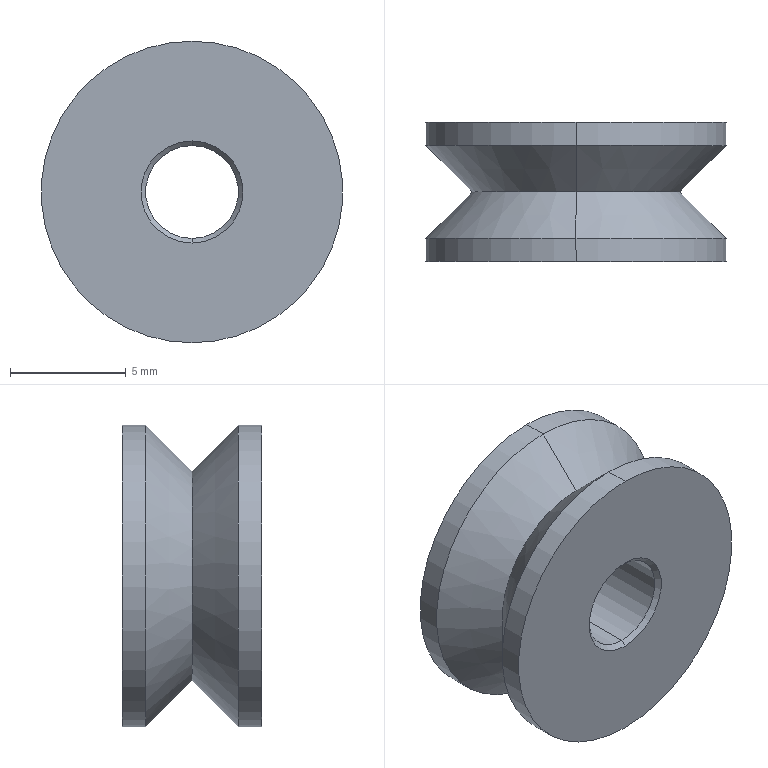Part | SolidWorks | features ICE 2, Blend 1, Chamfer 1, MirrorPattern 1 | 1 solid | 16 faces | box 13 x 6 x 13 mm | volume 573.868 mm3 | cone 8 | cylinder 6 | plane 2 | commonest cylinder face diameters 13 x4 4 x2
STEP:
#1=CARTESIAN_POINT('',(0.,-2.8,2.));
#2=VERTEX_POINT('',#1);
#3=CARTESIAN_POINT('',(0.,-2.8,-2.));
#4=VERTEX_POINT('',#3);
#5=CARTESIAN_POINT('',(0.,-2.8,0.));
#6=DIRECTION('',(0.,-1.,0.));
#7=DIRECTION('',(0.,0.,-1.));
#8=AXIS2_PLACEMENT_3D('',#5,#6,#7);
#9=CIRCLE('',#8,2.);
#10=EDGE_CURVE('',#2,#4,#9,.T.);
#11=ORIENTED_EDGE('',*,*,#10,.F.);
#12=CARTESIAN_POINT('',(0.,-3.,2.2));
#13=VERTEX_POINT('',#12);
#14=CARTESIAN_POINT('',(0.,-3.,2.2));
#15=DIRECTION('',(0.,-0.7071,0.7071));
#16=VECTOR('',#15,1000.);
#17=LINE('',#14,#16);
#18=EDGE_CURVE('',#2,#13,#17,.T.);
#19=ORIENTED_EDGE('',*,*,#18,.T.);
#20=CARTESIAN_POINT('',(0.,-3.,-2.2));
#21=VERTEX_POINT('',#20);
#22=CARTESIAN_POINT('',(0.,-3.,0.));
#23=DIRECTION('',(0.,1.,0.));
#24=DIRECTION('',(0.,0.,-1.));
#25=AXIS2_PLACEMENT_3D('',#22,#23,#24);
#26=CIRCLE('',#25,2.2);
#27=EDGE_CURVE('',#21,#13,#26,.T.);
#28=ORIENTED_EDGE('',*,*,#27,.F.);
#29=CARTESIAN_POINT('',(0.,-3.,-2.2));
#30=DIRECTION('',(0.,-0.7071,-0.7071));
#31=VECTOR('',#30,1000.);
#32=LINE('',#29,#31);
#33=EDGE_CURVE('',#4,#21,#32,.T.);
#34=ORIENTED_EDGE('',*,*,#33,.F.);
#35=EDGE_LOOP('',(#11,#19,#28,#34));
#36=FACE_OUTER_BOUND('',#35,.T.);
#37=CARTESIAN_POINT('',(0.,-3.,0.));
#38=DIRECTION('',(0.,-1.,0.));
#39=DIRECTION('',(0.,0.,-1.));
#40=AXIS2_PLACEMENT_3D('',#37,#38,#39);
#41=CONICAL_SURFACE('',#40,2.2,0.7854);
#42=ADVANCED_FACE('',(#36),#41,.F.);
#43=CARTESIAN_POINT('',(0.,2.8,-2.));
#44=VERTEX_POINT('',#43);
#45=CARTESIAN_POINT('',(0.,2.8,2.));
#46=VERTEX_POINT('',#45);
#47=CARTESIAN_POINT('',(0.,2.8,0.));
#48=DIRECTION('',(0.,1.,0.));
#49=DIRECTION('',(0.,0.,1.));
#50=AXIS2_PLACEMENT_3D('',#47,#48,#49);
#51=CIRCLE('',#50,2.);
#52=EDGE_CURVE('',#44,#46,#51,.T.);
#53=ORIENTED_EDGE('',*,*,#52,.F.);
#54=CARTESIAN_POINT('',(0.,3.,-2.2));
#55=VERTEX_POINT('',#54);
#56=CARTESIAN_POINT('',(0.,2.8,-2.));
#57=DIRECTION('',(0.,0.7071,-0.7071));
#58=VECTOR('',#57,1000.);
#59=LINE('',#56,#58);
#60=EDGE_CURVE('',#44,#55,#59,.T.);
#61=ORIENTED_EDGE('',*,*,#60,.T.);
#62=CARTESIAN_POINT('',(0.,3.,2.2));
#63=VERTEX_POINT('',#62);
#64=CARTESIAN_POINT('',(0.,3.,0.));
#65=DIRECTION('',(0.,-1.,0.));
#66=DIRECTION('',(0.,0.,1.));
#67=AXIS2_PLACEMENT_3D('',#64,#65,#66);
#68=CIRCLE('',#67,2.2);
#69=EDGE_CURVE('',#63,#55,#68,.T.);
#70=ORIENTED_EDGE('',*,*,#69,.F.);
#71=CARTESIAN_POINT('',(0.,2.8,2.));
#72=DIRECTION('',(0.,0.7071,0.7071));
#73=VECTOR('',#72,1000.);
#74=LINE('',#71,#73);
#75=EDGE_CURVE('',#46,#63,#74,.T.);
#76=ORIENTED_EDGE('',*,*,#75,.F.);
#77=EDGE_LOOP('',(#53,#61,#70,#76));
#78=FACE_OUTER_BOUND('',#77,.T.);
#79=CARTESIAN_POINT('',(0.,2.8,0.));
#80=DIRECTION('',(0.,1.,0.));
#81=DIRECTION('',(0.,0.,1.));
#82=AXIS2_PLACEMENT_3D('',#79,#80,#81);
#83=CONICAL_SURFACE('',#82,2.,0.7854);
#84=ADVANCED_FACE('',(#78),#83,.F.);
#85=ORIENTED_EDGE('',*,*,#10,.T.);
#86=CARTESIAN_POINT('',(0.,-3.,-2.));
#87=DIRECTION('',(0.,1.,0.));
#88=VECTOR('',#87,1000.);
#89=LINE('',#86,#88);
#90=EDGE_CURVE('',#4,#44,#89,.T.);
#91=ORIENTED_EDGE('',*,*,#90,.T.);
#92=ORIENTED_EDGE('',*,*,#52,.T.);
#93=CARTESIAN_POINT('',(0.,-3.,2.));
#94=DIRECTION('',(0.,1.,0.));
#95=VECTOR('',#94,1000.);
#96=LINE('',#93,#95);
#97=EDGE_CURVE('',#2,#46,#96,.T.);
#98=ORIENTED_EDGE('',*,*,#97,.F.);
#99=EDGE_LOOP('',(#85,#91,#92,#98));
#100=FACE_OUTER_BOUND('',#99,.T.);
#101=CARTESIAN_POINT('',(0.,-3.,0.));
#102=DIRECTION('',(0.,1.,0.));
#103=DIRECTION('',(0.,0.,1.));
#104=AXIS2_PLACEMENT_3D('',#101,#102,#103);
#105=CYLINDRICAL_SURFACE('',#104,2.);
#106=ADVANCED_FACE('',(#100),#105,.F.);
#107=CARTESIAN_POINT('',(0.,-3.,6.5));
#108=VERTEX_POINT('',#107);
#109=CARTESIAN_POINT('',(0.,-3.,-6.5));
#110=VERTEX_POINT('',#109);
#111=CARTESIAN_POINT('',(0.,-3.,0.));
#112=DIRECTION('',(0.,1.,0.));
#113=DIRECTION('',(0.,0.,1.));
#114=AXIS2_PLACEMENT_3D('',#111,#112,#113);
#115=CIRCLE('',#114,6.5);
#116=EDGE_CURVE('',#108,#110,#115,.T.);
#117=ORIENTED_EDGE('',*,*,#116,.T.);
#118=CARTESIAN_POINT('',(0.,-2.,-6.5));
#119=VERTEX_POINT('',#118);
#120=CARTESIAN_POINT('',(0.,-3.,-6.5));
#121=DIRECTION('',(0.,1.,0.));
#122=VECTOR('',#121,1000.);
#123=LINE('',#120,#122);
#124=EDGE_CURVE('',#110,#119,#123,.T.);
#125=ORIENTED_EDGE('',*,*,#124,.T.);
#126=CARTESIAN_POINT('',(0.,-2.,6.5));
#127=VERTEX_POINT('',#126);
#128=CARTESIAN_POINT('',(0.,-2.,0.));
#129=DIRECTION('',(0.,1.,0.));
#130=DIRECTION('',(0.,0.,1.));
#131=AXIS2_PLACEMENT_3D('',#128,#129,#130);
#132=CIRCLE('',#131,6.5);
#133=EDGE_CURVE('',#127,#119,#132,.T.);
#134=ORIENTED_EDGE('',*,*,#133,.F.);
#135=CARTESIAN_POINT('',(0.,-3.,6.5));
#136=DIRECTION('',(0.,1.,0.));
#137=VECTOR('',#136,1000.);
#138=LINE('',#135,#137);
#139=EDGE_CURVE('',#108,#127,#138,.T.);
#140=ORIENTED_EDGE('',*,*,#139,.F.);
#141=EDGE_LOOP('',(#117,#125,#134,#140));
#142=FACE_OUTER_BOUND('',#141,.T.);
#143=CARTESIAN_POINT('',(0.,-3.,0.));
#144=DIRECTION('',(0.,1.,0.));
#145=DIRECTION('',(0.,0.,1.));
#146=AXIS2_PLACEMENT_3D('',#143,#144,#145);
#147=CYLINDRICAL_SURFACE('',#146,6.5);
#148=ADVANCED_FACE('',(#142),#147,.T.);
#149=CARTESIAN_POINT('',(0.,0.,-4.5));
#150=VERTEX_POINT('',#149);
#151=CARTESIAN_POINT('',(0.,0.,4.5));
#152=VERTEX_POINT('',#151);
#153=CARTESIAN_POINT('',(0.,0.,0.));
#154=DIRECTION('',(0.,1.,0.));
#155=DIRECTION('',(0.,0.,1.));
#156=AXIS2_PLACEMENT_3D('',#153,#154,#155);
#157=CIRCLE('',#156,4.5);
#158=EDGE_CURVE('',#150,#152,#157,.T.);
#159=ORIENTED_EDGE('',*,*,#158,.F.);
#160=CARTESIAN_POINT('',(0.,0.,-4.5));
#161=DIRECTION('',(0.,-0.7071,-0.7071));
#162=VECTOR('',#161,1000.);
#163=LINE('',#160,#162);
#164=EDGE_CURVE('',#150,#119,#163,.T.);
#165=ORIENTED_EDGE('',*,*,#164,.T.);
#166=CARTESIAN_POINT('',(0.,-2.,0.));
#167=DIRECTION('',(0.,1.,0.));
#168=DIRECTION('',(0.,0.,1.));
#169=AXIS2_PLACEMENT_3D('',#166,#167,#168);
#170=CIRCLE('',#169,6.5);
#171=EDGE_CURVE('',#119,#127,#170,.T.);
#172=ORIENTED_EDGE('',*,*,#171,.T.);
#173=CARTESIAN_POINT('',(0.,0.,4.5));
#174=DIRECTION('',(0.,-0.7071,0.7071));
#175=VECTOR('',#174,1000.);
#176=LINE('',#173,#175);
#177=EDGE_CURVE('',#152,#127,#176,.T.);
#178=ORIENTED_EDGE('',*,*,#177,.F.);
#179=EDGE_LOOP('',(#159,#165,#172,#178));
#180=FACE_OUTER_BOUND('',#179,.T.);
#181=CARTESIAN_POINT('',(0.,0.,0.));
#182=DIRECTION('',(0.,-1.,0.));
#183=DIRECTION('',(0.,0.,1.));
#184=AXIS2_PLACEMENT_3D('',#181,#182,#183);
#185=CONICAL_SURFACE('',#184,4.5,0.7854);
#186=ADVANCED_FACE('',(#180),#185,.T.);
#187=CARTESIAN_POINT('',(0.,3.,6.5));
#188=VERTEX_POINT('',#187);
#189=CARTESIAN_POINT('',(0.,3.,-6.5));
#190=VERTEX_POINT('',#189);
#191=CARTESIAN_POINT('',(0.,3.,0.));
#192=DIRECTION('',(0.,1.,0.));
#193=DIRECTION('',(0.,0.,1.));
#194=AXIS2_PLACEMENT_3D('',#191,#192,#193);
#195=CIRCLE('',#194,6.5);
#196=EDGE_CURVE('',#188,#190,#195,.T.);
#197=ORIENTED_EDGE('',*,*,#196,.F.);
#198=CARTESIAN_POINT('',(0.,2.,6.5));
#199=VERTEX_POINT('',#198);
#200=CARTESIAN_POINT('',(0.,3.,6.5));
#201=DIRECTION('',(0.,-1.,0.));
#202=VECTOR('',#201,1000.);
#203=LINE('',#200,#202);
#204=EDGE_CURVE('',#188,#199,#203,.T.);
#205=ORIENTED_EDGE('',*,*,#204,.T.);
#206=CARTESIAN_POINT('',(0.,2.,-6.5));
#207=VERTEX_POINT('',#206);
#208=CARTESIAN_POINT('',(0.,2.,0.));
#209=DIRECTION('',(0.,1.,0.));
#210=DIRECTION('',(0.,0.,1.));
#211=AXIS2_PLACEMENT_3D('',#208,#209,#210);
#212=CIRCLE('',#211,6.5);
#213=EDGE_CURVE('',#199,#207,#212,.T.);
#214=ORIENTED_EDGE('',*,*,#213,.T.);
#215=CARTESIAN_POINT('',(0.,3.,-6.5));
#216=DIRECTION('',(0.,-1.,0.));
#217=VECTOR('',#216,1000.);
#218=LINE('',#215,#217);
#219=EDGE_CURVE('',#190,#207,#218,.T.);
#220=ORIENTED_EDGE('',*,*,#219,.F.);
#221=EDGE_LOOP('',(#197,#205,#214,#220));
#222=FACE_OUTER_BOUND('',#221,.T.);
#223=CARTESIAN_POINT('',(0.,3.,0.));
#224=DIRECTION('',(0.,-1.,0.));
#225=DIRECTION('',(0.,0.,-1.));
#226=AXIS2_PLACEMENT_3D('',#223,#224,#225);
#227=CYLINDRICAL_SURFACE('',#226,6.5);
#228=ADVANCED_FACE('',(#222),#227,.T.);
#229=CARTESIAN_POINT('',(0.,0.,0.));
#230=DIRECTION('',(0.,1.,0.));
#231=DIRECTION('',(0.,0.,1.));
#232=AXIS2_PLACEMENT_3D('',#229,#230,#231);
#233=CIRCLE('',#232,4.5);
#234=EDGE_CURVE('',#152,#150,#233,.T.);
#235=ORIENTED_EDGE('',*,*,#234,.T.);
#236=CARTESIAN_POINT('',(0.,0.,-4.5));
#237=DIRECTION('',(0.,0.7071,-0.7071));
#238=VECTOR('',#237,1000.);
#239=LINE('',#236,#238);
#240=EDGE_CURVE('',#150,#207,#239,.T.);
#241=ORIENTED_EDGE('',*,*,#240,.T.);
#242=ORIENTED_EDGE('',*,*,#213,.F.);
#243=CARTESIAN_POINT('',(0.,0.,4.5));
#244=DIRECTION('',(0.,0.7071,0.7071));
#245=VECTOR('',#244,1000.);
#246=LINE('',#243,#245);
#247=EDGE_CURVE('',#152,#199,#246,.T.);
#248=ORIENTED_EDGE('',*,*,#247,.F.);
#249=EDGE_LOOP('',(#235,#241,#242,#248));
#250=FACE_OUTER_BOUND('',#249,.T.);
#251=CARTESIAN_POINT('',(0.,0.,0.));
#252=DIRECTION('',(0.,1.,0.));
#253=DIRECTION('',(0.,0.,1.));
#254=AXIS2_PLACEMENT_3D('',#251,#252,#253);
#255=CONICAL_SURFACE('',#254,4.5,0.7854);
#256=ADVANCED_FACE('',(#250),#255,.T.);
#257=ORIENTED_EDGE('',*,*,#240,.F.);
#258=ORIENTED_EDGE('',*,*,#158,.T.);
#259=ORIENTED_EDGE('',*,*,#247,.T.);
#260=CARTESIAN_POINT('',(0.,2.,0.));
#261=DIRECTION('',(0.,1.,0.));
#262=DIRECTION('',(0.,0.,1.));
#263=AXIS2_PLACEMENT_3D('',#260,#261,#262);
#264=CIRCLE('',#263,6.5);
#265=EDGE_CURVE('',#207,#199,#264,.T.);
#266=ORIENTED_EDGE('',*,*,#265,.F.);
#267=EDGE_LOOP('',(#257,#258,#259,#266));
#268=FACE_OUTER_BOUND('',#267,.T.);
#269=CARTESIAN_POINT('',(0.,0.,0.));
#270=DIRECTION('',(0.,1.,0.));
#271=DIRECTION('',(0.,0.,1.));
#272=AXIS2_PLACEMENT_3D('',#269,#270,#271);
#273=CONICAL_SURFACE('',#272,4.5,0.7854);
#274=ADVANCED_FACE('',(#268),#273,.T.);
#275=ORIENTED_EDGE('',*,*,#204,.F.);
#276=CARTESIAN_POINT('',(0.,3.,0.));
#277=DIRECTION('',(0.,1.,0.));
#278=DIRECTION('',(0.,0.,1.));
#279=AXIS2_PLACEMENT_3D('',#276,#277,#278);
#280=CIRCLE('',#279,6.5);
#281=EDGE_CURVE('',#190,#188,#280,.T.);
#282=ORIENTED_EDGE('',*,*,#281,.F.);
#283=ORIENTED_EDGE('',*,*,#219,.T.);
#284=ORIENTED_EDGE('',*,*,#265,.T.);
#285=EDGE_LOOP('',(#275,#282,#283,#284));
#286=FACE_OUTER_BOUND('',#285,.T.);
#287=CARTESIAN_POINT('',(0.,3.,0.));
#288=DIRECTION('',(0.,-1.,0.));
#289=DIRECTION('',(0.,0.,-1.));
#290=AXIS2_PLACEMENT_3D('',#287,#288,#289);
#291=CYLINDRICAL_SURFACE('',#290,6.5);
#292=ADVANCED_FACE('',(#286),#291,.T.);
#293=ORIENTED_EDGE('',*,*,#69,.T.);
#294=CARTESIAN_POINT('',(0.,3.,0.));
#295=DIRECTION('',(0.,-1.,0.));
#296=DIRECTION('',(0.,0.,1.));
#297=AXIS2_PLACEMENT_3D('',#294,#295,#296);
#298=CIRCLE('',#297,2.2);
#299=EDGE_CURVE('',#55,#63,#298,.T.);
#300=ORIENTED_EDGE('',*,*,#299,.T.);
#301=EDGE_LOOP('',(#293,#300));
#302=FACE_BOUND('',#301,.T.);
#303=ORIENTED_EDGE('',*,*,#281,.T.);
#304=ORIENTED_EDGE('',*,*,#196,.T.);
#305=EDGE_LOOP('',(#303,#304));
#306=FACE_OUTER_BOUND('',#305,.T.);
#307=CARTESIAN_POINT('',(0.,3.,0.));
#308=DIRECTION('',(0.,1.,0.));
#309=DIRECTION('',(0.,0.,1.));
#310=AXIS2_PLACEMENT_3D('',#307,#308,#309);
#311=PLANE('',#310);
#312=ADVANCED_FACE('',(#302,#306),#311,.T.);
#313=ORIENTED_EDGE('',*,*,#164,.F.);
#314=ORIENTED_EDGE('',*,*,#234,.F.);
#315=ORIENTED_EDGE('',*,*,#177,.T.);
#316=ORIENTED_EDGE('',*,*,#133,.T.);
#317=EDGE_LOOP('',(#313,#314,#315,#316));
#318=FACE_OUTER_BOUND('',#317,.T.);
#319=CARTESIAN_POINT('',(0.,0.,0.));
#320=DIRECTION('',(0.,-1.,0.));
#321=DIRECTION('',(0.,0.,1.));
#322=AXIS2_PLACEMENT_3D('',#319,#320,#321);
#323=CONICAL_SURFACE('',#322,4.5,0.7854);
#324=ADVANCED_FACE('',(#318),#323,.T.);
#325=ORIENTED_EDGE('',*,*,#124,.F.);
#326=CARTESIAN_POINT('',(0.,-3.,0.));
#327=DIRECTION('',(0.,1.,0.));
#328=DIRECTION('',(0.,0.,1.));
#329=AXIS2_PLACEMENT_3D('',#326,#327,#328);
#330=CIRCLE('',#329,6.5);
#331=EDGE_CURVE('',#110,#108,#330,.T.);
#332=ORIENTED_EDGE('',*,*,#331,.T.);
#333=ORIENTED_EDGE('',*,*,#139,.T.);
#334=ORIENTED_EDGE('',*,*,#171,.F.);
#335=EDGE_LOOP('',(#325,#332,#333,#334));
#336=FACE_OUTER_BOUND('',#335,.T.);
#337=CARTESIAN_POINT('',(0.,-3.,0.));
#338=DIRECTION('',(0.,1.,0.));
#339=DIRECTION('',(0.,0.,1.));
#340=AXIS2_PLACEMENT_3D('',#337,#338,#339);
#341=CYLINDRICAL_SURFACE('',#340,6.5);
#342=ADVANCED_FACE('',(#336),#341,.T.);
#343=ORIENTED_EDGE('',*,*,#27,.T.);
#344=CARTESIAN_POINT('',(0.,-3.,0.));
#345=DIRECTION('',(0.,1.,0.));
#346=DIRECTION('',(0.,0.,-1.));
#347=AXIS2_PLACEMENT_3D('',#344,#345,#346);
#348=CIRCLE('',#347,2.2);
#349=EDGE_CURVE('',#13,#21,#348,.T.);
#350=ORIENTED_EDGE('',*,*,#349,.T.);
#351=EDGE_LOOP('',(#343,#350));
#352=FACE_BOUND('',#351,.T.);
#353=ORIENTED_EDGE('',*,*,#116,.F.);
#354=ORIENTED_EDGE('',*,*,#331,.F.);
#355=EDGE_LOOP('',(#353,#354));
#356=FACE_OUTER_BOUND('',#355,.T.);
#357=CARTESIAN_POINT('',(0.,-3.,0.));
#358=DIRECTION('',(0.,-1.,0.));
#359=DIRECTION('',(0.,0.,1.));
#360=AXIS2_PLACEMENT_3D('',#357,#358,#359);
#361=PLANE('',#360);
#362=ADVANCED_FACE('',(#352,#356),#361,.T.);
#363=ORIENTED_EDGE('',*,*,#90,.F.);
#364=CARTESIAN_POINT('',(0.,-2.8,0.));
#365=DIRECTION('',(0.,-1.,0.));
#366=DIRECTION('',(0.,0.,-1.));
#367=AXIS2_PLACEMENT_3D('',#364,#365,#366);
#368=CIRCLE('',#367,2.);
#369=EDGE_CURVE('',#4,#2,#368,.T.);
#370=ORIENTED_EDGE('',*,*,#369,.T.);
#371=ORIENTED_EDGE('',*,*,#97,.T.);
#372=CARTESIAN_POINT('',(0.,2.8,0.));
#373=DIRECTION('',(0.,1.,0.));
#374=DIRECTION('',(0.,0.,1.));
#375=AXIS2_PLACEMENT_3D('',#372,#373,#374);
#376=CIRCLE('',#375,2.);
#377=EDGE_CURVE('',#46,#44,#376,.T.);
#378=ORIENTED_EDGE('',*,*,#377,.T.);
#379=EDGE_LOOP('',(#363,#370,#371,#378));
#380=FACE_OUTER_BOUND('',#379,.T.);
#381=CARTESIAN_POINT('',(0.,-3.,0.));
#382=DIRECTION('',(0.,1.,0.));
#383=DIRECTION('',(0.,0.,1.));
#384=AXIS2_PLACEMENT_3D('',#381,#382,#383);
#385=CYLINDRICAL_SURFACE('',#384,2.);
#386=ADVANCED_FACE('',(#380),#385,.F.);
#387=ORIENTED_EDGE('',*,*,#60,.F.);
#388=ORIENTED_EDGE('',*,*,#377,.F.);
#389=ORIENTED_EDGE('',*,*,#75,.T.);
#390=ORIENTED_EDGE('',*,*,#299,.F.);
#391=EDGE_LOOP('',(#387,#388,#389,#390));
#392=FACE_OUTER_BOUND('',#391,.T.);
#393=CARTESIAN_POINT('',(0.,2.8,0.));
#394=DIRECTION('',(0.,1.,0.));
#395=DIRECTION('',(0.,0.,1.));
#396=AXIS2_PLACEMENT_3D('',#393,#394,#395);
#397=CONICAL_SURFACE('',#396,2.,0.7854);
#398=ADVANCED_FACE('',(#392),#397,.F.);
#399=ORIENTED_EDGE('',*,*,#18,.F.);
#400=ORIENTED_EDGE('',*,*,#369,.F.);
#401=ORIENTED_EDGE('',*,*,#33,.T.);
#402=ORIENTED_EDGE('',*,*,#349,.F.);
#403=EDGE_LOOP('',(#399,#400,#401,#402));
#404=FACE_OUTER_BOUND('',#403,.T.);
#405=CARTESIAN_POINT('',(0.,-3.,0.));
#406=DIRECTION('',(0.,-1.,0.));
#407=DIRECTION('',(0.,0.,-1.));
#408=AXIS2_PLACEMENT_3D('',#405,#406,#407);
#409=CONICAL_SURFACE('',#408,2.2,0.7854);
#410=ADVANCED_FACE('',(#404),#409,.F.);
#411=CLOSED_SHELL('',(#42,#84,#106,#148,#186,#228,#256,#274,#292,#312,#324,#342,#362,#386,#398,#410));
#412=MANIFOLD_SOLID_BREP('',#411);
#413=CARTESIAN_POINT('',(0.,0.,0.));
#414=DIRECTION('',(0.,0.,1.));
#415=DIRECTION('',(1.,0.,0.));
#416=AXIS2_PLACEMENT_3D('',#413,#414,#415);
#417=(LENGTH_UNIT()NAMED_UNIT(*)SI_UNIT(.MILLI.,.METRE.));
#418=UNCERTAINTY_MEASURE_WITH_UNIT(LENGTH_MEASURE(0.00001),#417,'','');
#419=(NAMED_UNIT(*)PLANE_ANGLE_UNIT()SI_UNIT($,.RADIAN.));
#420=(NAMED_UNIT(*)SI_UNIT($,.STERADIAN.)SOLID_ANGLE_UNIT());
#421=(GEOMETRIC_REPRESENTATION_CONTEXT(3)GLOBAL_UNCERTAINTY_ASSIGNED_CONTEXT((#418))GLOBAL_UNIT_ASSIGNED_CONTEXT((#417,#419,#420))REPRESENTATION_CONTEXT('',''));
#422=ADVANCED_BREP_SHAPE_REPRESENTATION('',(#412,#416),#421);